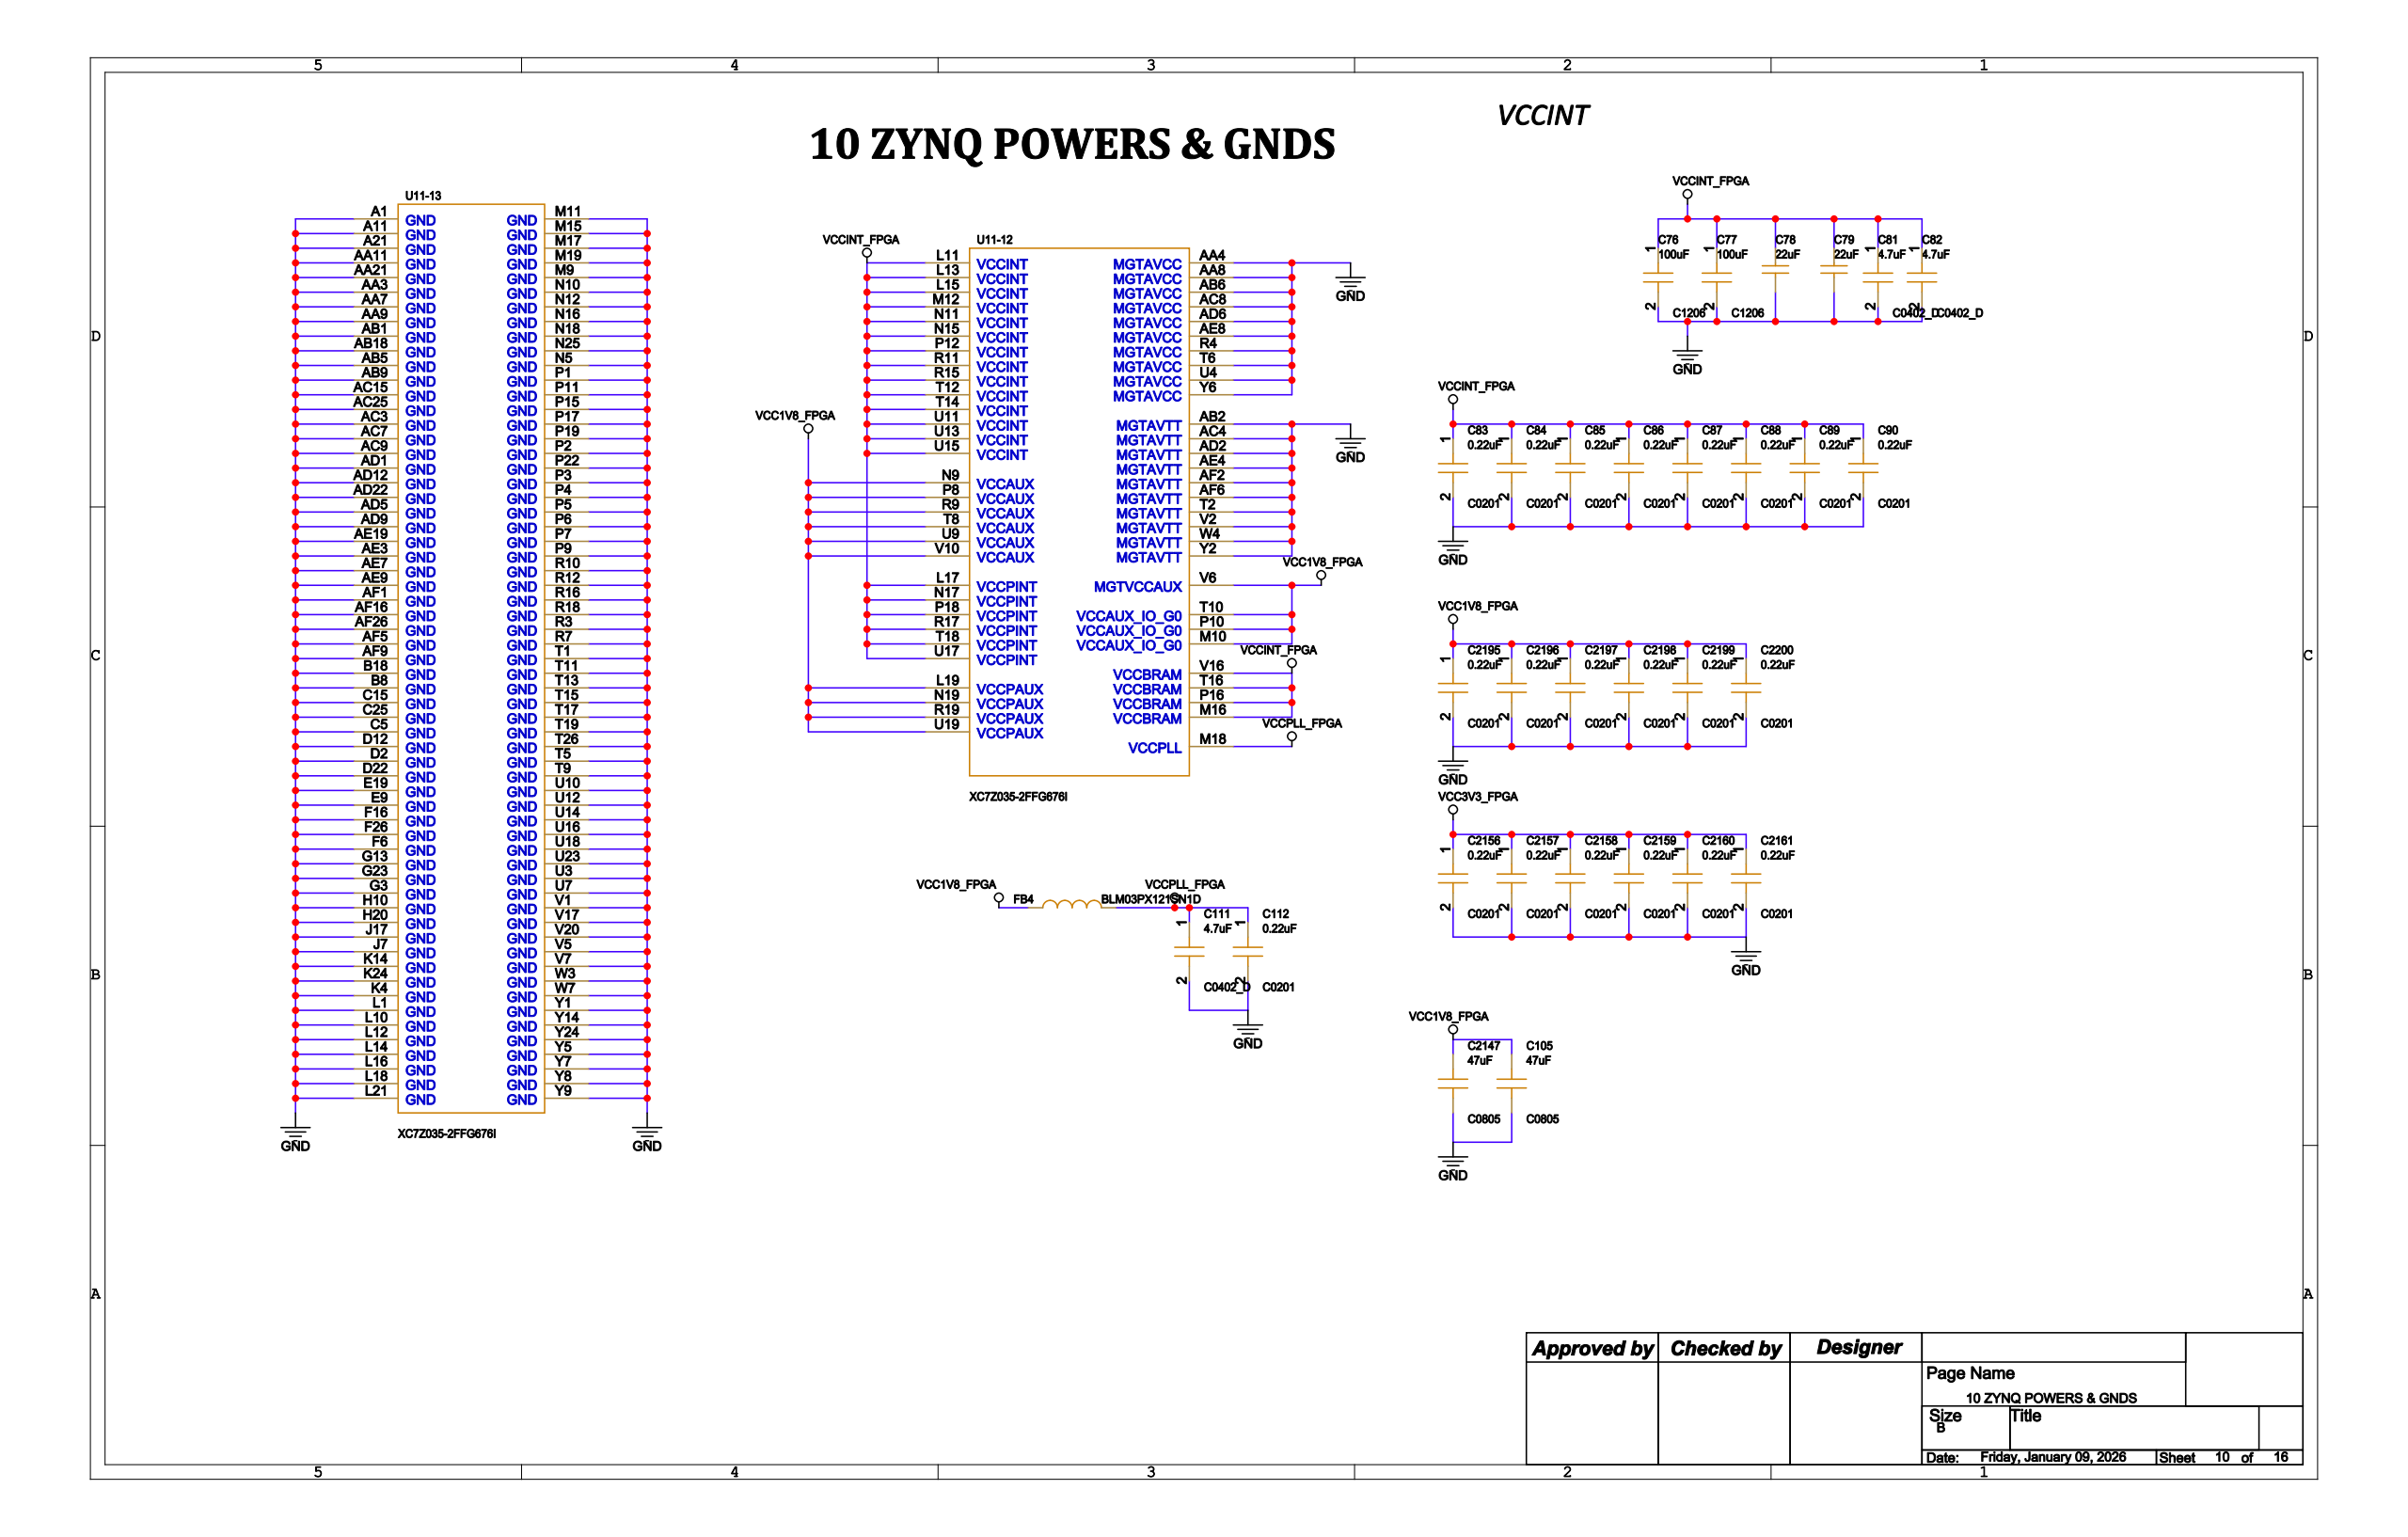Circuit board | Cadence Allegro | 442 parts | 326 nets | one sheet of the schematic
Parts on this sheet (reference | value | footprint):
C76 | 100uF | C1206
C77 | 100uF | C1206
C78 | 22uF | C0805
C79 | 22uF | C0805
C81 | 4.7uF | C0402_D
C82 | 4.7uF | C0402_D
C83 | 0.22uF | C0201
C84 | 0.22uF | C0201
C85 | 0.22uF | C0201
C86 | 0.22uF | C0201
C87 | 0.22uF | C0201
C88 | 0.22uF | C0201
C89 | 0.22uF | C0201
C90 | 0.22uF | C0201
C105 | 47uF | C0805
C111 | 4.7uF | C0402_D
C112 | 0.22uF | C0201
C2147 | 47uF | C0805
C2156 | 0.22uF | C0201
C2157 | 0.22uF | C0201
C2158 | 0.22uF | C0201
C2159 | 0.22uF | C0201
C2160 | 0.22uF | C0201
C2161 | 0.22uF | C0201
C2195 | 0.22uF | C0201
C2196 | 0.22uF | C0201
C2197 | 0.22uF | C0201
C2198 | 0.22uF | C0201
C2199 | 0.22uF | C0201
C2200 | 0.22uF | C0201
FB4 | BLM03PX121SN1D | L0201
U11 | XC7Z035-2FFG676I | FPGA_ZYNQ7045_676
U14 | MT41K256M16TW-107 | FBGA_DDR4_96P
Nets of these parts (net: part-pin ...):
GND: C76-2 C77-2 C78-2 C79-2 C81-2 C82-2 C83-2 C84-2 C85-2 C86-2 C87-2 C88-2 C89-2 C90-2 C105-2 C111-2 C112-2 C2147-2 C2156-2 C2157-2 C2158-2 C2159-2 C2160-2 C2161-2 C2195-2 C2196-2 C2197-2 C2198-2 C2199-2 C2200-2 U11-A1 U11-A11 U11-A21 U11-AA3 U11-AA4 U11-AA7 U11-AA8 U11-AA9 U11-AA11 U11-AA21 U11-AB1 U11-AB2 U11-AB5 U11-AB6 U11-AB9 U11-AB18 U11-AC3 U11-AC4 U11-AC7 U11-AC8 U11-AC9 U11-AC15 U11-AC25 U11-AD1 U11-AD2 U11-AD5 U11-AD6 U11-AD9 U11-AD12 U11-AD22 U11-AE3 U11-AE4 U11-AE7 U11-AE8 U11-AE9 U11-AE19 U11-AF1 U11-AF2 U11-AF5 U11-AF6 U11-AF9 U11-AF16 U11-AF26 U11-B8 U11-B18 U11-C5 U11-C15 U11-C25 U11-D2 U11-D12 U11-D22 U11-E9 U11-E19 U11-F6 U11-F16 U11-F26 U11-G3 U11-G13 U11-G23 U11-H10 U11-H20 U11-J7 U11-J17 U11-K4 U11-K14 U11-K24 U11-L1 U11-L10 U11-L12 U11-L14 U11-L16 U11-L18 U11-L21 U11-M9 U11-M11 U11-M15 U11-M17 U11-M19 U11-N5 U11-N10 U11-N12 U11-N16 U11-N18 U11-N25 U11-P1 U11-P2 U11-P3 U11-P4 U11-P5 U11-P6 U11-P7 U11-P9 U11-P11 U11-P15 U11-P17 U11-P19 U11-P22 U11-R3 U11-R4 U11-R7 U11-R10 U11-R12 U11-R16 U11-R18 U11-T1 U11-T2 U11-T5 U11-T6 U11-T9 U11-T11 U11-T13 U11-T15 U11-T17 U11-T19 U11-T26 U11-U3 U11-U4 U11-U7 U11-U10 U11-U12 U11-U14 U11-U16 U11-U18 U11-U23 U11-V1 U11-V2 U11-V5 U11-V7 U11-V17 U11-V20 U11-W3 U11-W4 U11-W7 U11-Y1 U11-Y2 U11-Y5 U11-Y6 U11-Y7 U11-Y8 U11-Y9 U11-Y14 U11-Y24 U14-M9 U14-P1 U14-P9 U14-T1 U14-T9
VCC1V8_FPGA: C105-1 C2147-1 C2195-1 C2196-1 C2197-1 C2198-1 C2199-1 C2200-1 FB4-1 U11-L19 U11-M10 U11-N9 U11-N19 U11-P8 U11-P10 U11-R9 U11-R19 U11-T8 U11-T10 U11-U9 U11-U19 U11-V6 U11-V10
VCCPLL_FPGA: C111-1 C112-1 FB4-2 U11-M18
VCCINT_FPGA: C76-1 C77-1 C78-1 C79-1 C81-1 C82-1 C83-1 C84-1 C85-1 C86-1 C87-1 C88-1 C89-1 C90-1 U11-L11 U11-L13 U11-L15 U11-L17 U11-M12 U11-M16 U11-N11 U11-N15 U11-N17 U11-P12 U11-P16 U11-P18 U11-R11 U11-R15 U11-R17 U11-T12 U11-T14 U11-T16 U11-T18 U11-U11 U11-U13 U11-U15 U11-U17 U11-V16
VCC3V3_FPGA: C2156-1 C2157-1 C2158-1 C2159-1 C2160-1 C2161-1